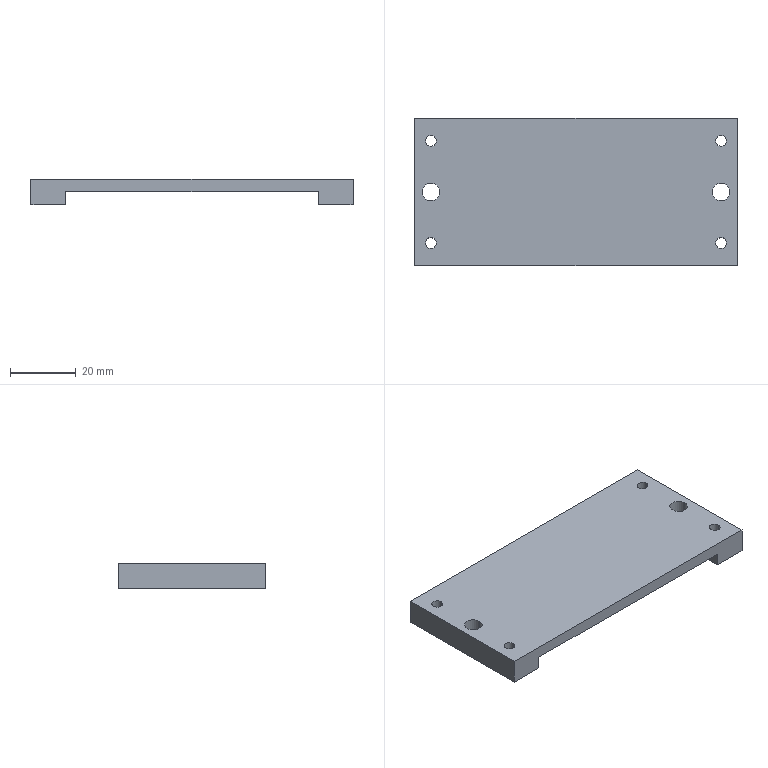Part | STEP file | 1 solid | 22 faces | box 97.7 x 44.7 x 7.7 mm | volume 19346 mm3 | cylinder 12 | plane 10 | commonest cylinder face diameters 3.3 x8 5.3 x4